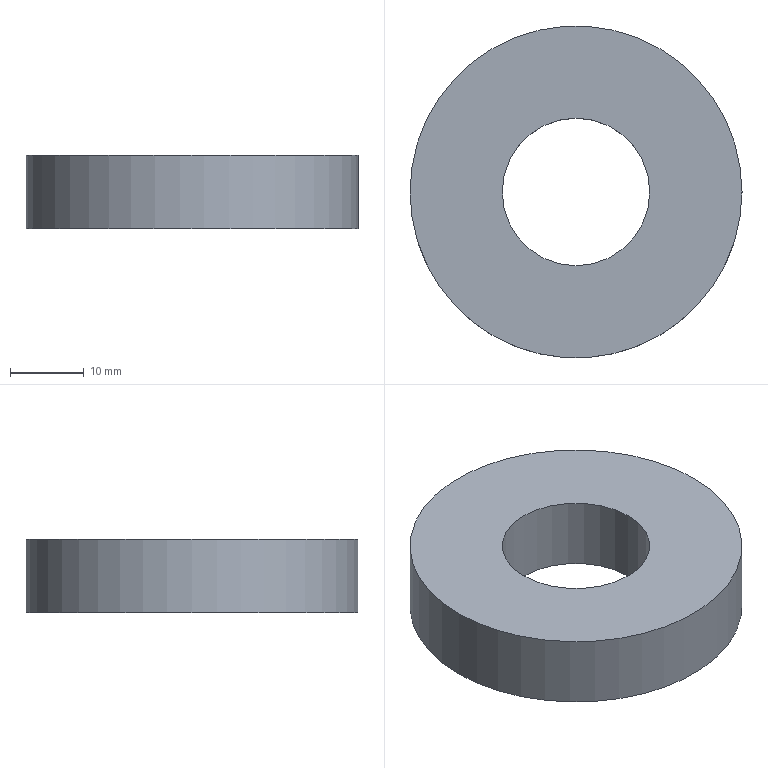Part | NX | features DATUM_CSYS 2, EXTRUDE 1, SKETCH 1 | 1 solid | 4 faces | box 45 x 45 x 10 mm | volume 12763 mm3 | cylinder 2 | plane 2 | commonest cylinder face diameters 20 x1 45 x1
STEP:
#1=CARTESIAN_POINT('',(22.5,0.,10.));
#2=VERTEX_POINT('',#1);
#3=CARTESIAN_POINT('',(0.,0.,10.));
#4=DIRECTION('',(0.,0.,1.));
#5=DIRECTION('',(1.,0.,0.));
#6=AXIS2_PLACEMENT_3D('',#3,#4,#5);
#7=CIRCLE('',#6,22.5);
#8=EDGE_CURVE('',#2,#2,#7,.T.);
#9=ORIENTED_EDGE('',*,*,#8,.F.);
#10=EDGE_LOOP('',(#9));
#11=FACE_BOUND('',#10,.T.);
#12=CARTESIAN_POINT('',(22.5,0.,0.));
#13=VERTEX_POINT('',#12);
#14=CARTESIAN_POINT('',(0.,0.,0.));
#15=DIRECTION('',(0.,0.,1.));
#16=DIRECTION('',(1.,0.,0.));
#17=AXIS2_PLACEMENT_3D('',#14,#15,#16);
#18=CIRCLE('',#17,22.5);
#19=EDGE_CURVE('',#13,#13,#18,.T.);
#20=ORIENTED_EDGE('',*,*,#19,.T.);
#21=EDGE_LOOP('',(#20));
#22=FACE_BOUND('',#21,.T.);
#23=CARTESIAN_POINT('',(0.,0.,10.));
#24=DIRECTION('',(0.,0.,-1.));
#25=DIRECTION('',(-1.,0.,0.));
#26=AXIS2_PLACEMENT_3D('',#23,#24,#25);
#27=CYLINDRICAL_SURFACE('',#26,22.5);
#28=ADVANCED_FACE('',(#11,#22),#27,.T.);
#29=CARTESIAN_POINT('',(10.,0.,10.));
#30=VERTEX_POINT('',#29);
#31=CARTESIAN_POINT('',(0.,0.,10.));
#32=DIRECTION('',(0.,0.,1.));
#33=DIRECTION('',(1.,0.,0.));
#34=AXIS2_PLACEMENT_3D('',#31,#32,#33);
#35=CIRCLE('',#34,10.);
#36=EDGE_CURVE('',#30,#30,#35,.T.);
#37=ORIENTED_EDGE('',*,*,#36,.T.);
#38=EDGE_LOOP('',(#37));
#39=FACE_BOUND('',#38,.T.);
#40=CARTESIAN_POINT('',(10.,0.,0.));
#41=VERTEX_POINT('',#40);
#42=CARTESIAN_POINT('',(0.,0.,0.));
#43=DIRECTION('',(0.,0.,1.));
#44=DIRECTION('',(1.,0.,0.));
#45=AXIS2_PLACEMENT_3D('',#42,#43,#44);
#46=CIRCLE('',#45,10.);
#47=EDGE_CURVE('',#41,#41,#46,.T.);
#48=ORIENTED_EDGE('',*,*,#47,.F.);
#49=EDGE_LOOP('',(#48));
#50=FACE_BOUND('',#49,.T.);
#51=CARTESIAN_POINT('',(0.,0.,10.));
#52=DIRECTION('',(0.,0.,-1.));
#53=DIRECTION('',(-1.,0.,0.));
#54=AXIS2_PLACEMENT_3D('',#51,#52,#53);
#55=CYLINDRICAL_SURFACE('',#54,10.);
#56=ADVANCED_FACE('',(#39,#50),#55,.F.);
#57=ORIENTED_EDGE('',*,*,#8,.T.);
#58=EDGE_LOOP('',(#57));
#59=FACE_BOUND('',#58,.T.);
#60=ORIENTED_EDGE('',*,*,#36,.F.);
#61=EDGE_LOOP('',(#60));
#62=FACE_BOUND('',#61,.T.);
#63=CARTESIAN_POINT('',(0.,0.,10.));
#64=DIRECTION('',(0.,0.,1.));
#65=DIRECTION('',(1.,0.,0.));
#66=AXIS2_PLACEMENT_3D('',#63,#64,#65);
#67=PLANE('',#66);
#68=ADVANCED_FACE('',(#59,#62),#67,.T.);
#69=ORIENTED_EDGE('',*,*,#19,.F.);
#70=EDGE_LOOP('',(#69));
#71=FACE_BOUND('',#70,.T.);
#72=ORIENTED_EDGE('',*,*,#47,.T.);
#73=EDGE_LOOP('',(#72));
#74=FACE_BOUND('',#73,.T.);
#75=CARTESIAN_POINT('',(0.,0.,0.));
#76=DIRECTION('',(0.,0.,1.));
#77=DIRECTION('',(1.,0.,0.));
#78=AXIS2_PLACEMENT_3D('',#75,#76,#77);
#79=PLANE('',#78);
#80=ADVANCED_FACE('',(#71,#74),#79,.F.);
#81=CLOSED_SHELL('',(#28,#56,#68,#80));
#82=MANIFOLD_SOLID_BREP('',#81);
#83=(LENGTH_UNIT()NAMED_UNIT(*)SI_UNIT(.MILLI.,.METRE.));
#84=UNCERTAINTY_MEASURE_WITH_UNIT(LENGTH_MEASURE(0.00001),#83,'','');
#85=(NAMED_UNIT(*)PLANE_ANGLE_UNIT()SI_UNIT($,.RADIAN.));
#86=(NAMED_UNIT(*)SI_UNIT($,.STERADIAN.)SOLID_ANGLE_UNIT());
#87=(GEOMETRIC_REPRESENTATION_CONTEXT(3)GLOBAL_UNCERTAINTY_ASSIGNED_CONTEXT((#84))GLOBAL_UNIT_ASSIGNED_CONTEXT((#83,#85,#86))REPRESENTATION_CONTEXT('',''));
#88=ADVANCED_BREP_SHAPE_REPRESENTATION('',(#82),#87);